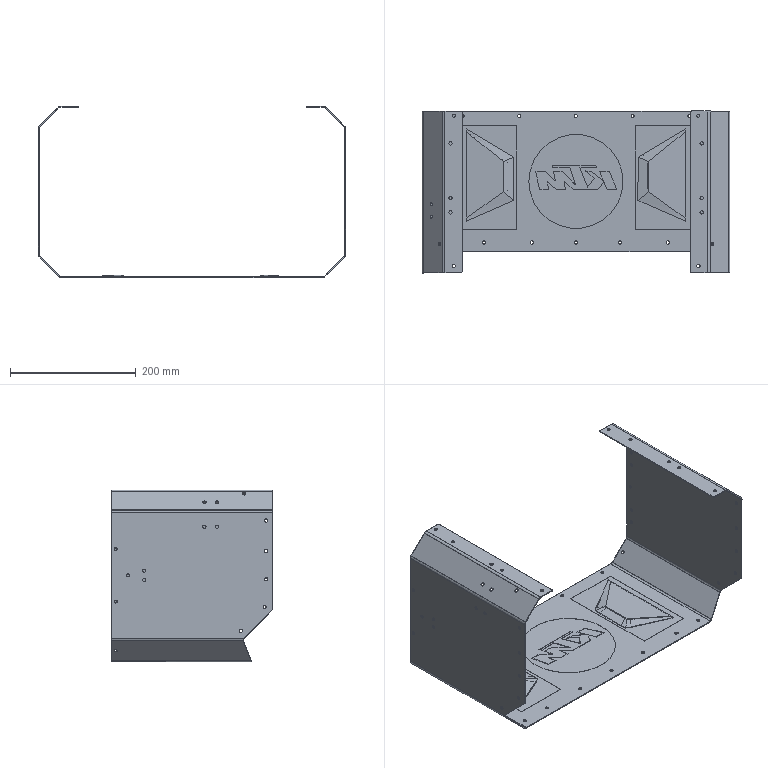Part | SolidWorks | features BaseBody 1 | 1 solid | 279 faces | box 490.179 x 258.012 x 273.944 mm | volume 368834 mm3 | cylinder 130 | spline 77 | plane 72 | commonest cylinder face diameters 5.2 x70 4.9 x30 10 x8 13 x8 4 x6 1.905 x3